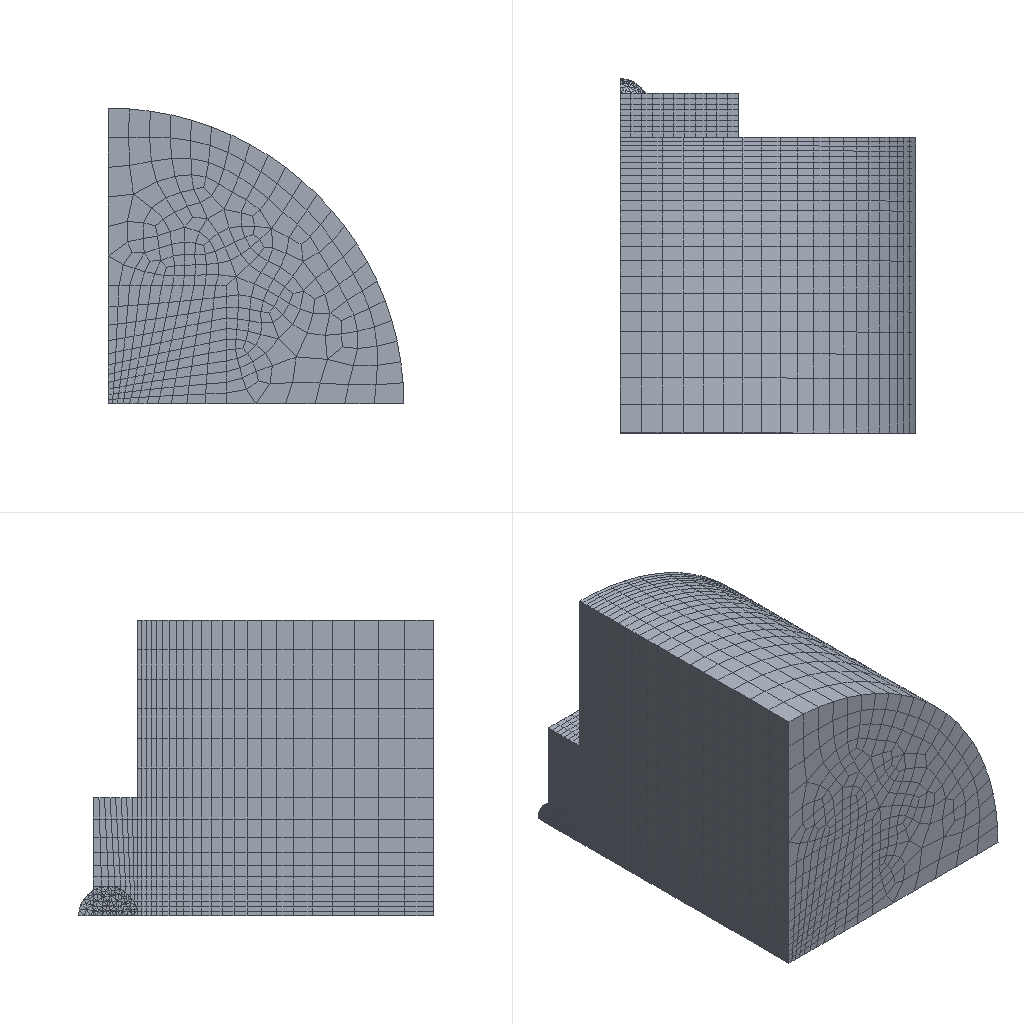Simulation study | abaqus
Set-up summary:
category,name,step,type,value,unit,region
solver,abaqus
solver,version,,,Abaqus/Explicit 2020
units,not stated in the deck,,not stated
analysis,deck,,dynamic temperature-displacement,dynamic temperature-displacement
load_step,Step-1,Step-1,dynamic temperature-displacement
load_step,requested,,,1
mesh,nodes,,,10266
mesh,elements,,,10038
element_type,C3D4T,,solid,1319
element_type,EC3D8RT,,solid,8719
load,load commands in deck,,count,1
bc,support commands in deck,,count,7
material,AL,,in results
material,MG,,in results
check,setup vs results,,match,"per instance, exact: element labels, types and connectivity; labels of the nodes the elements use; coordinates of those nodes at SINGLE_PRECISION in 2 of 2 instance(s)"
Abaqus input file, long lists of numbers shortened:
*Heading
** Job name: Job-2 Model name: Model-1
** Generated by: Abaqus/CAE 2020
*Preprint, echo=NO, model=NO, history=NO, contact=NO
**
** PARTS
**
*Part, name=oula
*Node
      1, 0.04, 0.015,           0.
      2, 0.04, 0.015, 0.04
** (9934 more lines like these left out)
*Element, type=EC3D8RT
  1,  101,  552, 2417,  412,    1,   14,  272,   47
  2,  552,  553, 2418, 2417,   14,   15,  273,  272
** (8717 more lines like these left out)
*Nset, nset=Set-31, generate
    1,  9936,     1
*Elset, elset=Set-31, generate
    1,  8719,     1
** Section: oula
*Eulerian Section, elset=Set-31
mg, mg-1
*Surface, type=EULERIAN MATERIAL, name=mg-1
mg-1
*End Part
**
*Part, name=work-2
*Node
      1, 0.01, 0.01,           0.
      2,           0.,           0.,           0.
** (328 more lines like these left out)
*Element, type=C3D4T
   1, 192, 193, 194, 195
   2, 192, 196,  74, 197
** (1317 more lines like these left out)
*Nset, nset=Set-3, generate
   1,  330,    1
*Elset, elset=Set-3, generate
    1,  1319,     1
** Section: al
*Solid Section, elset=Set-3, material=al
,
*End Part
**
**
** ASSEMBLY
**
*Assembly, name=Assembly
**
*Instance, name=work-2-1, part=work-2
*End Instance
**
*Instance, name=oula-1, part=oula
*End Instance
**
*Nset, nset=Set-1, instance=oula-1
    3,    4,    6,    7,    9,   10,   11,   12,   13,   31,   32,   33,   34,   35,   36,   37
   38,   39,   40,   65,   66,   67,   68,   69,   70,   71,   72,   73,   74,   82,   83,   84
** (547 more lines like these left out)
*Elset, elset=Set-1, instance=oula-1, generate
  969,  8719,     1
*Nset, nset=Set-2, instance=work-2-1, generate
   1,  330,    1
*Elset, elset=Set-2, instance=work-2-1, generate
    1,  1319,     1
*Nset, nset=Set-3, instance=oula-1, generate
    1,  9936,     1
*Elset, elset=Set-3, instance=oula-1, generate
    1,  8719,     1
*Nset, nset=Set-4, instance=work-2-1, generate
   1,  330,    1
*Elset, elset=Set-4, instance=work-2-1, generate
    1,  1319,     1
*Nset, nset=Set-5, instance=oula-1
    1,    4,    7,    8,   10,   12,   13,   41,   42,   43,   44,   45,   46,   47,   75,   76
   77,   78,   79,   80,   81,   82,   83,   84,   85,   86,   87,   88,   89,   90,   91,   92
** (31 more lines like these left out)
*Elset, elset=Set-5, instance=oula-1
    1,   12,   23,   34,   45,   56,   67,   78,   89,  100,  111,  122,  133,  144,  155,  166
  177,  188,  199,  210,  221,  232,  243,  254,  265,  276,  287,  298,  309,  320,  331,  342
** (28 more lines like these left out)
*Nset, nset=Set-6, instance=oula-1
    5,    6,    7,    8,    9,   11,   12,   48,   49,   50,   51,   52,   53,   54,   55,   56
   57,   58,   59,   60,   61,   62,   63,   64,   65,   66,   67,   68,   69,   70,   71,   72
** (31 more lines like these left out)
*Elset, elset=Set-6, instance=oula-1
  881,  882,  883,  884,  885,  886,  887,  888,  889,  890,  891,  892,  893,  894,  895,  896
  897,  898,  899,  900,  901,  902,  903,  904,  905,  906,  907,  908,  909,  910,  911,  912
** (28 more lines like these left out)
*Nset, nset=Set-7, instance=oula-1
   11,   12,   13,  219,  220,  221,  222,  223,  224,  225,  226,  227,  228,  229,  230,  231
  232,  233,  234,  235,  236,  237,  238,  239,  240,  241,  242,  243,  244,  245,  246,  247
** (21 more lines like these left out)
*Elset, elset=Set-7, instance=oula-1, generate
 8383,  8719,     1
*End Assembly
**
** MATERIALS
**
*Material, name=al
*Conductivity
247.,
*Density
 2.7e-09,
*Elastic
62000., 0.33
*Plastic
250.,0.
*Specific Heat
 9e+08,
*Material, name=mg
*Conductivity
156.,
*Density
 1.8e-09,
*Elastic
45000., 0.33
*Plastic
280.,0.
*Specific Heat
 1.02e+08,
**
** INTERACTION PROPERTIES
**
*Surface Interaction, name=IntProp-1
*Friction
 0.3,
*Surface Behavior, pressure-overclosure=HARD
**
** PREDEFINED FIELDS
**
** Name: Predefined Field-1   Type: Material assignment
*Initial Conditions, type=VOLUME FRACTION
Set-1, oula-1.mg-1, 1.
** Name: Predefined Field-2   Type: Temperature
*Initial Conditions, type=TEMPERATURE
Set-2, 623.
** Name: Predefined Field-3   Type: Temperature
*Initial Conditions, type=TEMPERATURE
Set-3, 298.
** Name: Predefined Field-4   Type: Velocity
*Initial Conditions, type=VELOCITY
Set-4, 1, 0.
Set-4, 2, -270000.
Set-4, 3, 0.
** ----------------------------------------------------------------
**
** STEP: Step-1
**
*Step, name=Step-1, nlgeom=YES
*Dynamic Temperature-displacement, Explicit
, 6e-08
*Bulk Viscosity
0.06, 1.2
** Mass Scaling: Semi-Automatic
**               Whole Model
*Fixed Mass Scaling, factor=50.
**
** BOUNDARY CONDITIONS
**
** Name: BC-1 Type: 速度/角速度
*Boundary, type=VELOCITY
Set-5, 3, 3
Set-5, 4, 4
Set-5, 5, 5
** Name: BC-2 Type: 速度/角速度
*Boundary, type=VELOCITY
Set-6, 1, 1
Set-6, 5, 5
Set-6, 6, 6
** Name: BC-3 Type: 速度/角速度
*Boundary, type=VELOCITY
Set-7, 2, 2
**
** INTERACTIONS
**
** Interaction: Int-1
*Contact, op=NEW
*Contact Inclusions, ALL EXTERIOR
*Contact Property Assignment
 ,  , IntProp-1
**
** OUTPUT REQUESTS
**
*Restart, write, number interval=1, time marks=NO
**
** FIELD OUTPUT: F-Output-1
**
*Output, field, number interval=50
*Node Output
A, NT, RF, RFL, RM, RT, U, V
*Element Output, directions=YES
DENSITY, E, ESDV, EVF, EVOL, FV, HFL, LE, MISES, MISESMAX, MISESONLY, PE, PEEQ, PEEQMAX, PEEQVAVG, PEMAG
PEVAVG, PRESSONLY, S, SDV, SSAVG, SVAVG, SVOL, TEMP, YIELDPOT
*Contact Output
CDISP, CSTRESS
**
** HISTORY OUTPUT: H-Output-1
**
*Output, history, variable=PRESELECT
*End Step
Results summary:
result,step,Step-1,completed,increments=394 time=5.99999978589949e-08/5.99999978589949e-08
result,analysis,,,"dynamic temperature-displacement, explict"
result,last_loadstep,,,1
result,primary field,,,"U, NT11"
result,reaction total,,FX,-0.009175,model units
result,reaction total,,FY,0.2564,model units
result,reaction total,,FZ,-0.00972,model units